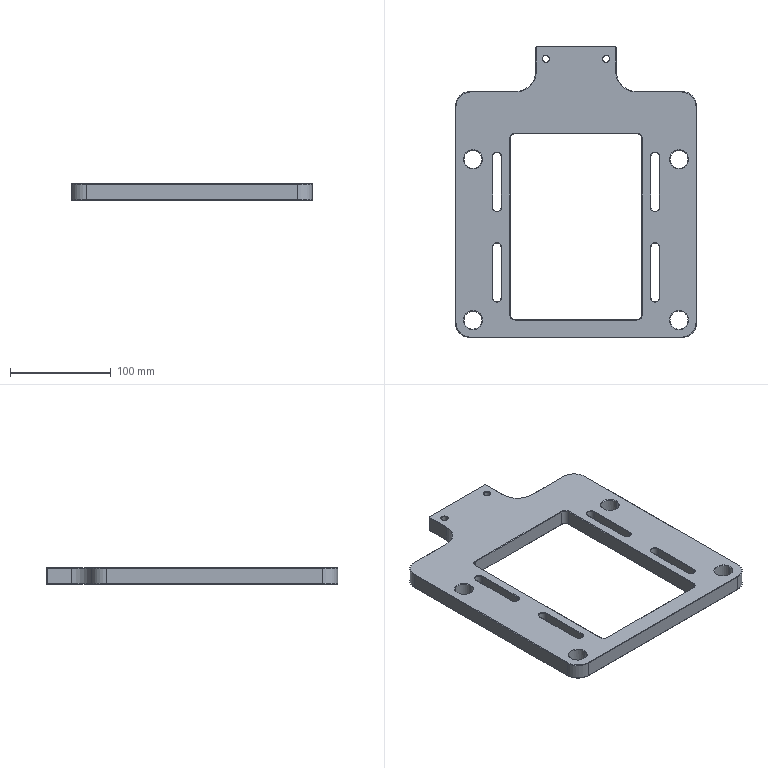Part | SolidWorks | features BaseBody 1 | 1 solid | 158 faces | box 240 x 290 x 16 mm | volume 561839 mm3 | plane 68 | cone 60 | cylinder 30 | commonest cylinder face diameters 8.5 x8 18 x8 6.5 x4 10 x4 30 x4 40 x2